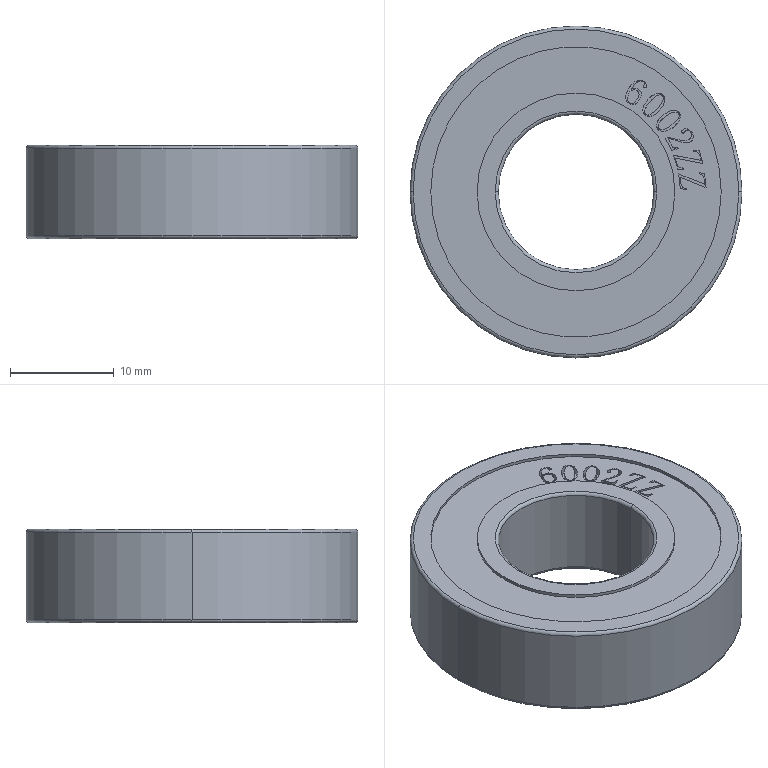Part | STEP file | Domestic single-row deep groove ball bearing NSK 6002ZZ-1 | 1 solid | 107 faces | box 32 x 32 x 9 mm | volume 5439 mm3 | spline 47 | plane 40 | cylinder 12 | torus 8 | commonest cylinder face diameters 19.067 x4 28 x4 15 x2 32 x2